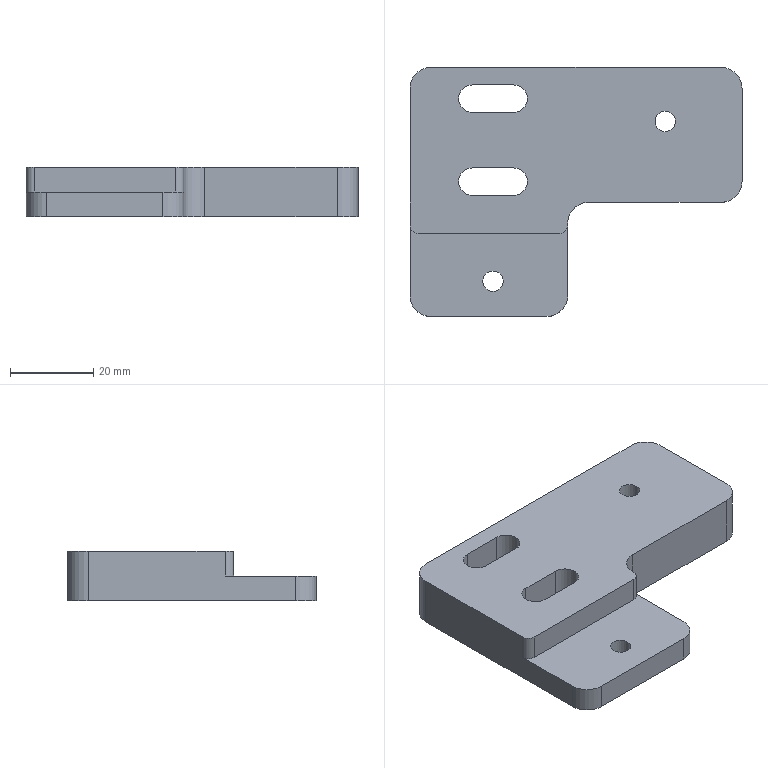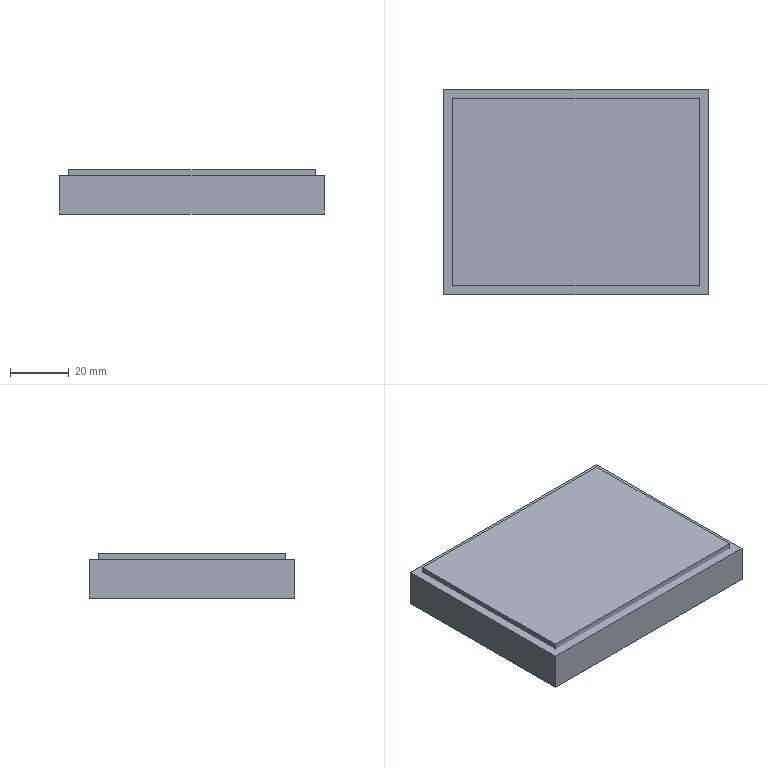CAM job | NX | 3-axis milling, drilling | part box 80 x 60 x 12 mm | stock box 90 x 70 x 15 mm
Tools:
number,name,description,diameter,corner_radius,flute_length,length,flutes
19,D80,Milling Tool-5 Parameters,80.0,0.0,50.0,75.0,2
15,D10,Milling Tool-5 Parameters,10.0,0.0,50.0,75.0,2
14,D10JING,Milling Tool-5 Parameters,10.0,0.0,50.0,75.0,2
11,D4,Milling Tool-5 Parameters,4.0,0.0,50.0,75.0,2
1,D6A45,Milling Tool-5 Parameters,6.0,0.0,50.0,75.0,2
5,5.0ZT,Drilling Tool,4.9,0.0,35.0,50.0,2
Operations:
program,operation,operation_type,tool,method,geometry_group,spindle_rpm,surface_speed,feed_per_tooth,feed_cut,feed_plunge,cut_length_mm,path_length_mm,cut_time_min,machine_time_min
1,FLOOR_WALL,VolumeBased25DMillingOperation,D80,METHOD,A,6500.0,1633.0,0.1154,1500.0,100.0,182.0,236.0,0.1213,0.1267
1,ADAPTIVE_MILLING,CavityMilling,D10,METHOD,A,9500.0,298.0,0.1842,3500.0,1000.0,8453.343,8762.881,2.42,2.45
1,FACE_MILLING,FaceMilling,D10,METHOD,A,9500.0,298.0,0.1842,3500.0,1000.0,1884.038,2063.489,0.5511,0.5691
1,ZLEVEL_PROFILE_COPY_1,ZLevelMilling,D10JING,METHOD,A,9500.0,298.0,0.0632,1200.0,1000.0,557.989,626.989,0.508,0.5149
1,FLOOR_WALL_2,VolumeBased25DMillingOperation,D10JING,METHOD,A,9500.0,298.0,0.0789,1500.0,100.0,284.409,472.552,0.1896,0.2084
1,ZLEVEL_PROFILE,ZLevelMilling,D4,METHOD,A,9500.0,119.0,0.0868,1650.0,100.0,1806.38,1965.283,1.095,1.111
1,DRILLING,Operation,D6A45,METHOD,A,5000.0,94.0,0.035,350.0,0.0,8.0,142.319,0.0229,0.0363
1,DRILLING_COPY_COPY_COPY,Operation,5.0ZT,METHOD,A,2000.0,26.0,0.075,300.0,0.0,29.944,185.576,0.0998,0.1154
1,PLANAR_MILL_COPY_COPY_COPY,PlanarMilling,D6A45,METHOD,A,9500.0,179.0,0.0658,1250.0,100.0,335.683,658.481,0.2685,0.3008
1,PLANAR_MILL_COPY_COPY_COPY_COPY,PlanarMilling,D6A45,METHOD,A,9500.0,179.0,0.0658,1250.0,100.0,94.552,260.506,0.0756,0.0922
2,FLOOR_WALL_COPY,VolumeBased25DMillingOperation,D80,METHOD,B,6500.0,1633.0,0.1154,1500.0,100.0,528.0,1024.001,0.352,0.4016
2,PLANAR_MILL_COPY_COPY_COPY_COPY_1,PlanarMilling,D6A45,METHOD,B,9500.0,179.0,0.0658,1250.0,100.0,387.995,776.511,0.3104,0.3492